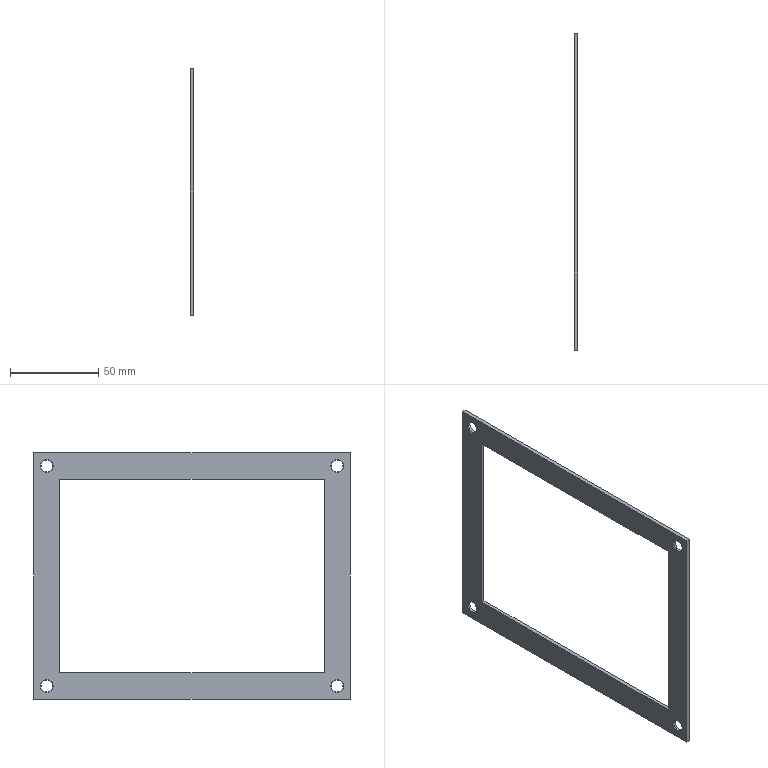Part | NX | 1 solid | 22 faces | box 2 x 180 x 140 mm | volume 17112 mm3 | plane 10 | cone 8 | cylinder 4 | commonest cylinder face diameters 6.6 x4
STEP:
#1=CARTESIAN_POINT('',(0.,-75.,-55.));
#2=VERTEX_POINT('',#1);
#3=CARTESIAN_POINT('',(0.,-75.,55.));
#4=VERTEX_POINT('',#3);
#5=CARTESIAN_POINT('',(0.,-75.,-55.));
#6=DIRECTION('',(0.,0.,1.));
#7=VECTOR('',#6,1.);
#8=LINE('',#5,#7);
#9=EDGE_CURVE('',#2,#4,#8,.T.);
#10=ORIENTED_EDGE('',*,*,#9,.T.);
#11=CARTESIAN_POINT('',(2.,-75.,55.));
#12=VERTEX_POINT('',#11);
#13=CARTESIAN_POINT('',(2.,-75.,55.));
#14=DIRECTION('',(-1.,0.,0.));
#15=VECTOR('',#14,1.);
#16=LINE('',#13,#15);
#17=EDGE_CURVE('',#12,#4,#16,.T.);
#18=ORIENTED_EDGE('',*,*,#17,.F.);
#19=CARTESIAN_POINT('',(2.,-75.,-55.));
#20=VERTEX_POINT('',#19);
#21=CARTESIAN_POINT('',(2.,-75.,-55.));
#22=DIRECTION('',(0.,0.,1.));
#23=VECTOR('',#22,1.);
#24=LINE('',#21,#23);
#25=EDGE_CURVE('',#20,#12,#24,.T.);
#26=ORIENTED_EDGE('',*,*,#25,.F.);
#27=CARTESIAN_POINT('',(2.,-75.,-55.));
#28=DIRECTION('',(-1.,0.,0.));
#29=VECTOR('',#28,1.);
#30=LINE('',#27,#29);
#31=EDGE_CURVE('',#20,#2,#30,.T.);
#32=ORIENTED_EDGE('',*,*,#31,.T.);
#33=EDGE_LOOP('',(#10,#18,#26,#32));
#34=FACE_OUTER_BOUND('',#33,.T.);
#35=CARTESIAN_POINT('',(2.,-75.,-55.));
#36=DIRECTION('',(0.,-1.,0.));
#37=DIRECTION('',(0.,0.,1.));
#38=AXIS2_PLACEMENT_3D('',#35,#36,#37);
#39=PLANE('',#38);
#40=ADVANCED_FACE('',(#34),#39,.F.);
#41=CARTESIAN_POINT('',(0.,75.,55.));
#42=VERTEX_POINT('',#41);
#43=CARTESIAN_POINT('',(0.,-75.,55.));
#44=DIRECTION('',(0.,1.,0.));
#45=VECTOR('',#44,1.);
#46=LINE('',#43,#45);
#47=EDGE_CURVE('',#4,#42,#46,.T.);
#48=ORIENTED_EDGE('',*,*,#47,.T.);
#49=CARTESIAN_POINT('',(2.,75.,55.));
#50=VERTEX_POINT('',#49);
#51=CARTESIAN_POINT('',(2.,75.,55.));
#52=DIRECTION('',(-1.,0.,0.));
#53=VECTOR('',#52,1.);
#54=LINE('',#51,#53);
#55=EDGE_CURVE('',#50,#42,#54,.T.);
#56=ORIENTED_EDGE('',*,*,#55,.F.);
#57=CARTESIAN_POINT('',(2.,-75.,55.));
#58=DIRECTION('',(0.,1.,0.));
#59=VECTOR('',#58,1.);
#60=LINE('',#57,#59);
#61=EDGE_CURVE('',#12,#50,#60,.T.);
#62=ORIENTED_EDGE('',*,*,#61,.F.);
#63=ORIENTED_EDGE('',*,*,#17,.T.);
#64=EDGE_LOOP('',(#48,#56,#62,#63));
#65=FACE_OUTER_BOUND('',#64,.T.);
#66=CARTESIAN_POINT('',(2.,-75.,55.));
#67=DIRECTION('',(0.,0.,1.));
#68=DIRECTION('',(0.,1.,0.));
#69=AXIS2_PLACEMENT_3D('',#66,#67,#68);
#70=PLANE('',#69);
#71=ADVANCED_FACE('',(#65),#70,.F.);
#72=CARTESIAN_POINT('',(0.,75.,-55.));
#73=VERTEX_POINT('',#72);
#74=CARTESIAN_POINT('',(0.,75.,55.));
#75=DIRECTION('',(0.,0.,-1.));
#76=VECTOR('',#75,1.);
#77=LINE('',#74,#76);
#78=EDGE_CURVE('',#42,#73,#77,.T.);
#79=ORIENTED_EDGE('',*,*,#78,.T.);
#80=CARTESIAN_POINT('',(2.,75.,-55.));
#81=VERTEX_POINT('',#80);
#82=CARTESIAN_POINT('',(2.,75.,-55.));
#83=DIRECTION('',(-1.,0.,0.));
#84=VECTOR('',#83,1.);
#85=LINE('',#82,#84);
#86=EDGE_CURVE('',#81,#73,#85,.T.);
#87=ORIENTED_EDGE('',*,*,#86,.F.);
#88=CARTESIAN_POINT('',(2.,75.,55.));
#89=DIRECTION('',(0.,0.,-1.));
#90=VECTOR('',#89,1.);
#91=LINE('',#88,#90);
#92=EDGE_CURVE('',#50,#81,#91,.T.);
#93=ORIENTED_EDGE('',*,*,#92,.F.);
#94=ORIENTED_EDGE('',*,*,#55,.T.);
#95=EDGE_LOOP('',(#79,#87,#93,#94));
#96=FACE_OUTER_BOUND('',#95,.T.);
#97=CARTESIAN_POINT('',(2.,75.,55.));
#98=DIRECTION('',(0.,1.,0.));
#99=DIRECTION('',(0.,0.,-1.));
#100=AXIS2_PLACEMENT_3D('',#97,#98,#99);
#101=PLANE('',#100);
#102=ADVANCED_FACE('',(#96),#101,.F.);
#103=CARTESIAN_POINT('',(0.,-90.,70.));
#104=VERTEX_POINT('',#103);
#105=CARTESIAN_POINT('',(0.,-90.,-70.));
#106=VERTEX_POINT('',#105);
#107=CARTESIAN_POINT('',(0.,-90.,70.));
#108=DIRECTION('',(0.,0.,-1.));
#109=VECTOR('',#108,1.);
#110=LINE('',#107,#109);
#111=EDGE_CURVE('',#104,#106,#110,.T.);
#112=ORIENTED_EDGE('',*,*,#111,.T.);
#113=CARTESIAN_POINT('',(2.,-90.,-70.));
#114=VERTEX_POINT('',#113);
#115=CARTESIAN_POINT('',(2.,-90.,-70.));
#116=DIRECTION('',(-1.,0.,0.));
#117=VECTOR('',#116,1.);
#118=LINE('',#115,#117);
#119=EDGE_CURVE('',#114,#106,#118,.T.);
#120=ORIENTED_EDGE('',*,*,#119,.F.);
#121=CARTESIAN_POINT('',(2.,-90.,70.));
#122=VERTEX_POINT('',#121);
#123=CARTESIAN_POINT('',(2.,-90.,70.));
#124=DIRECTION('',(0.,0.,-1.));
#125=VECTOR('',#124,1.);
#126=LINE('',#123,#125);
#127=EDGE_CURVE('',#122,#114,#126,.T.);
#128=ORIENTED_EDGE('',*,*,#127,.F.);
#129=CARTESIAN_POINT('',(2.,-90.,70.));
#130=DIRECTION('',(-1.,0.,0.));
#131=VECTOR('',#130,1.);
#132=LINE('',#129,#131);
#133=EDGE_CURVE('',#122,#104,#132,.T.);
#134=ORIENTED_EDGE('',*,*,#133,.T.);
#135=EDGE_LOOP('',(#112,#120,#128,#134));
#136=FACE_OUTER_BOUND('',#135,.T.);
#137=CARTESIAN_POINT('',(2.,-90.,70.));
#138=DIRECTION('',(0.,1.,0.));
#139=DIRECTION('',(0.,0.,-1.));
#140=AXIS2_PLACEMENT_3D('',#137,#138,#139);
#141=PLANE('',#140);
#142=ADVANCED_FACE('',(#136),#141,.F.);
#143=CARTESIAN_POINT('',(0.,90.,-70.));
#144=VERTEX_POINT('',#143);
#145=CARTESIAN_POINT('',(0.,-90.,-70.));
#146=DIRECTION('',(0.,1.,0.));
#147=VECTOR('',#146,1.);
#148=LINE('',#145,#147);
#149=EDGE_CURVE('',#106,#144,#148,.T.);
#150=ORIENTED_EDGE('',*,*,#149,.T.);
#151=CARTESIAN_POINT('',(2.,90.,-70.));
#152=VERTEX_POINT('',#151);
#153=CARTESIAN_POINT('',(2.,90.,-70.));
#154=DIRECTION('',(-1.,0.,0.));
#155=VECTOR('',#154,1.);
#156=LINE('',#153,#155);
#157=EDGE_CURVE('',#152,#144,#156,.T.);
#158=ORIENTED_EDGE('',*,*,#157,.F.);
#159=CARTESIAN_POINT('',(2.,-90.,-70.));
#160=DIRECTION('',(0.,1.,0.));
#161=VECTOR('',#160,1.);
#162=LINE('',#159,#161);
#163=EDGE_CURVE('',#114,#152,#162,.T.);
#164=ORIENTED_EDGE('',*,*,#163,.F.);
#165=ORIENTED_EDGE('',*,*,#119,.T.);
#166=EDGE_LOOP('',(#150,#158,#164,#165));
#167=FACE_OUTER_BOUND('',#166,.T.);
#168=CARTESIAN_POINT('',(2.,-90.,-70.));
#169=DIRECTION('',(0.,0.,1.));
#170=DIRECTION('',(0.,1.,0.));
#171=AXIS2_PLACEMENT_3D('',#168,#169,#170);
#172=PLANE('',#171);
#173=ADVANCED_FACE('',(#167),#172,.F.);
#174=CARTESIAN_POINT('',(0.,90.,70.));
#175=VERTEX_POINT('',#174);
#176=CARTESIAN_POINT('',(0.,90.,-70.));
#177=DIRECTION('',(0.,0.,1.));
#178=VECTOR('',#177,1.);
#179=LINE('',#176,#178);
#180=EDGE_CURVE('',#144,#175,#179,.T.);
#181=ORIENTED_EDGE('',*,*,#180,.T.);
#182=CARTESIAN_POINT('',(2.,90.,70.));
#183=VERTEX_POINT('',#182);
#184=CARTESIAN_POINT('',(2.,90.,70.));
#185=DIRECTION('',(-1.,0.,0.));
#186=VECTOR('',#185,1.);
#187=LINE('',#184,#186);
#188=EDGE_CURVE('',#183,#175,#187,.T.);
#189=ORIENTED_EDGE('',*,*,#188,.F.);
#190=CARTESIAN_POINT('',(2.,90.,-70.));
#191=DIRECTION('',(0.,0.,1.));
#192=VECTOR('',#191,1.);
#193=LINE('',#190,#192);
#194=EDGE_CURVE('',#152,#183,#193,.T.);
#195=ORIENTED_EDGE('',*,*,#194,.F.);
#196=ORIENTED_EDGE('',*,*,#157,.T.);
#197=EDGE_LOOP('',(#181,#189,#195,#196));
#198=FACE_OUTER_BOUND('',#197,.T.);
#199=CARTESIAN_POINT('',(2.,90.,-70.));
#200=DIRECTION('',(0.,-1.,0.));
#201=DIRECTION('',(0.,0.,1.));
#202=AXIS2_PLACEMENT_3D('',#199,#200,#201);
#203=PLANE('',#202);
#204=ADVANCED_FACE('',(#198),#203,.F.);
#205=CARTESIAN_POINT('',(0.,90.,70.));
#206=DIRECTION('',(0.,-1.,0.));
#207=VECTOR('',#206,1.);
#208=LINE('',#205,#207);
#209=EDGE_CURVE('',#175,#104,#208,.T.);
#210=ORIENTED_EDGE('',*,*,#209,.T.);
#211=ORIENTED_EDGE('',*,*,#133,.F.);
#212=CARTESIAN_POINT('',(2.,90.,70.));
#213=DIRECTION('',(0.,-1.,0.));
#214=VECTOR('',#213,1.);
#215=LINE('',#212,#214);
#216=EDGE_CURVE('',#183,#122,#215,.T.);
#217=ORIENTED_EDGE('',*,*,#216,.F.);
#218=ORIENTED_EDGE('',*,*,#188,.T.);
#219=EDGE_LOOP('',(#210,#211,#217,#218));
#220=FACE_OUTER_BOUND('',#219,.T.);
#221=CARTESIAN_POINT('',(2.,90.,70.));
#222=DIRECTION('',(0.,0.,-1.));
#223=DIRECTION('',(0.,-1.,0.));
#224=AXIS2_PLACEMENT_3D('',#221,#222,#223);
#225=PLANE('',#224);
#226=ADVANCED_FACE('',(#220),#225,.F.);
#227=CARTESIAN_POINT('',(0.,75.,-55.));
#228=DIRECTION('',(0.,-1.,0.));
#229=VECTOR('',#228,1.);
#230=LINE('',#227,#229);
#231=EDGE_CURVE('',#73,#2,#230,.T.);
#232=ORIENTED_EDGE('',*,*,#231,.T.);
#233=ORIENTED_EDGE('',*,*,#31,.F.);
#234=CARTESIAN_POINT('',(2.,75.,-55.));
#235=DIRECTION('',(0.,-1.,0.));
#236=VECTOR('',#235,1.);
#237=LINE('',#234,#236);
#238=EDGE_CURVE('',#81,#20,#237,.T.);
#239=ORIENTED_EDGE('',*,*,#238,.F.);
#240=ORIENTED_EDGE('',*,*,#86,.T.);
#241=EDGE_LOOP('',(#232,#233,#239,#240));
#242=FACE_OUTER_BOUND('',#241,.T.);
#243=CARTESIAN_POINT('',(2.,75.,-55.));
#244=DIRECTION('',(0.,0.,-1.));
#245=DIRECTION('',(0.,-1.,0.));
#246=AXIS2_PLACEMENT_3D('',#243,#244,#245);
#247=PLANE('',#246);
#248=ADVANCED_FACE('',(#242),#247,.F.);
#249=CARTESIAN_POINT('',(2.,82.5,58.8));
#250=VERTEX_POINT('',#249);
#251=CARTESIAN_POINT('',(2.,82.5,62.5));
#252=DIRECTION('',(-1.,0.,0.));
#253=DIRECTION('',(0.,0.,-1.));
#254=AXIS2_PLACEMENT_3D('',#251,#252,#253);
#255=CIRCLE('',#254,3.7);
#256=EDGE_CURVE('',#250,#250,#255,.T.);
#257=ORIENTED_EDGE('',*,*,#256,.T.);
#258=EDGE_LOOP('',(#257));
#259=FACE_BOUND('',#258,.T.);
#260=CARTESIAN_POINT('',(2.,82.5,-66.2));
#261=VERTEX_POINT('',#260);
#262=CARTESIAN_POINT('',(2.,82.5,-62.5));
#263=DIRECTION('',(-1.,0.,0.));
#264=DIRECTION('',(0.,0.,-1.));
#265=AXIS2_PLACEMENT_3D('',#262,#263,#264);
#266=CIRCLE('',#265,3.7);
#267=EDGE_CURVE('',#261,#261,#266,.T.);
#268=ORIENTED_EDGE('',*,*,#267,.T.);
#269=EDGE_LOOP('',(#268));
#270=FACE_BOUND('',#269,.T.);
#271=CARTESIAN_POINT('',(2.,-82.5,58.8));
#272=VERTEX_POINT('',#271);
#273=CARTESIAN_POINT('',(2.,-82.5,62.5));
#274=DIRECTION('',(-1.,0.,0.));
#275=DIRECTION('',(0.,0.,-1.));
#276=AXIS2_PLACEMENT_3D('',#273,#274,#275);
#277=CIRCLE('',#276,3.7);
#278=EDGE_CURVE('',#272,#272,#277,.T.);
#279=ORIENTED_EDGE('',*,*,#278,.T.);
#280=EDGE_LOOP('',(#279));
#281=FACE_BOUND('',#280,.T.);
#282=CARTESIAN_POINT('',(2.,-82.5,-66.2));
#283=VERTEX_POINT('',#282);
#284=CARTESIAN_POINT('',(2.,-82.5,-62.5));
#285=DIRECTION('',(-1.,0.,0.));
#286=DIRECTION('',(0.,0.,-1.));
#287=AXIS2_PLACEMENT_3D('',#284,#285,#286);
#288=CIRCLE('',#287,3.7);
#289=EDGE_CURVE('',#283,#283,#288,.T.);
#290=ORIENTED_EDGE('',*,*,#289,.T.);
#291=EDGE_LOOP('',(#290));
#292=FACE_BOUND('',#291,.T.);
#293=ORIENTED_EDGE('',*,*,#127,.T.);
#294=ORIENTED_EDGE('',*,*,#163,.T.);
#295=ORIENTED_EDGE('',*,*,#194,.T.);
#296=ORIENTED_EDGE('',*,*,#216,.T.);
#297=EDGE_LOOP('',(#293,#294,#295,#296));
#298=FACE_BOUND('',#297,.T.);
#299=ORIENTED_EDGE('',*,*,#25,.T.);
#300=ORIENTED_EDGE('',*,*,#61,.T.);
#301=ORIENTED_EDGE('',*,*,#92,.T.);
#302=ORIENTED_EDGE('',*,*,#238,.T.);
#303=EDGE_LOOP('',(#299,#300,#301,#302));
#304=FACE_BOUND('',#303,.T.);
#305=CARTESIAN_POINT('',(2.,0.,0.));
#306=DIRECTION('',(1.,0.,0.));
#307=DIRECTION('',(0.,0.,1.));
#308=AXIS2_PLACEMENT_3D('',#305,#306,#307);
#309=PLANE('',#308);
#310=ADVANCED_FACE('',(#259,#270,#281,#292,#298,#304),#309,.T.);
#311=CARTESIAN_POINT('',(0.,82.5,58.8));
#312=VERTEX_POINT('',#311);
#313=CARTESIAN_POINT('',(0.,82.5,62.5));
#314=DIRECTION('',(1.,0.,0.));
#315=DIRECTION('',(0.,0.,-1.));
#316=AXIS2_PLACEMENT_3D('',#313,#314,#315);
#317=CIRCLE('',#316,3.7);
#318=EDGE_CURVE('',#312,#312,#317,.T.);
#319=ORIENTED_EDGE('',*,*,#318,.T.);
#320=EDGE_LOOP('',(#319));
#321=FACE_BOUND('',#320,.T.);
#322=CARTESIAN_POINT('',(0.,82.5,-66.2));
#323=VERTEX_POINT('',#322);
#324=CARTESIAN_POINT('',(0.,82.5,-62.5));
#325=DIRECTION('',(1.,0.,0.));
#326=DIRECTION('',(0.,0.,-1.));
#327=AXIS2_PLACEMENT_3D('',#324,#325,#326);
#328=CIRCLE('',#327,3.7);
#329=EDGE_CURVE('',#323,#323,#328,.T.);
#330=ORIENTED_EDGE('',*,*,#329,.T.);
#331=EDGE_LOOP('',(#330));
#332=FACE_BOUND('',#331,.T.);
#333=CARTESIAN_POINT('',(0.,-82.5,58.8));
#334=VERTEX_POINT('',#333);
#335=CARTESIAN_POINT('',(0.,-82.5,62.5));
#336=DIRECTION('',(1.,0.,0.));
#337=DIRECTION('',(0.,0.,-1.));
#338=AXIS2_PLACEMENT_3D('',#335,#336,#337);
#339=CIRCLE('',#338,3.7);
#340=EDGE_CURVE('',#334,#334,#339,.T.);
#341=ORIENTED_EDGE('',*,*,#340,.T.);
#342=EDGE_LOOP('',(#341));
#343=FACE_BOUND('',#342,.T.);
#344=CARTESIAN_POINT('',(0.,-82.5,-66.2));
#345=VERTEX_POINT('',#344);
#346=CARTESIAN_POINT('',(0.,-82.5,-62.5));
#347=DIRECTION('',(1.,0.,0.));
#348=DIRECTION('',(0.,0.,-1.));
#349=AXIS2_PLACEMENT_3D('',#346,#347,#348);
#350=CIRCLE('',#349,3.7);
#351=EDGE_CURVE('',#345,#345,#350,.T.);
#352=ORIENTED_EDGE('',*,*,#351,.T.);
#353=EDGE_LOOP('',(#352));
#354=FACE_BOUND('',#353,.T.);
#355=ORIENTED_EDGE('',*,*,#111,.F.);
#356=ORIENTED_EDGE('',*,*,#209,.F.);
#357=ORIENTED_EDGE('',*,*,#180,.F.);
#358=ORIENTED_EDGE('',*,*,#149,.F.);
#359=EDGE_LOOP('',(#355,#356,#357,#358));
#360=FACE_BOUND('',#359,.T.);
#361=ORIENTED_EDGE('',*,*,#9,.F.);
#362=ORIENTED_EDGE('',*,*,#231,.F.);
#363=ORIENTED_EDGE('',*,*,#78,.F.);
#364=ORIENTED_EDGE('',*,*,#47,.F.);
#365=EDGE_LOOP('',(#361,#362,#363,#364));
#366=FACE_BOUND('',#365,.T.);
#367=CARTESIAN_POINT('',(0.,0.,0.));
#368=DIRECTION('',(1.,0.,0.));
#369=DIRECTION('',(0.,0.,1.));
#370=AXIS2_PLACEMENT_3D('',#367,#368,#369);
#371=PLANE('',#370);
#372=ADVANCED_FACE('',(#321,#332,#343,#354,#360,#366),#371,.F.);
#373=CARTESIAN_POINT('',(1.6,-82.5,-65.8));
#374=VERTEX_POINT('',#373);
#375=CARTESIAN_POINT('',(1.6,-82.5,-62.5));
#376=DIRECTION('',(1.,0.,0.));
#377=DIRECTION('',(0.,0.,-1.));
#378=AXIS2_PLACEMENT_3D('',#375,#376,#377);
#379=CIRCLE('',#378,3.3);
#380=EDGE_CURVE('',#374,#374,#379,.T.);
#381=ORIENTED_EDGE('',*,*,#380,.T.);
#382=EDGE_LOOP('',(#381));
#383=FACE_BOUND('',#382,.T.);
#384=CARTESIAN_POINT('',(0.4,-82.5,-65.8));
#385=VERTEX_POINT('',#384);
#386=CARTESIAN_POINT('',(0.4,-82.5,-62.5));
#387=DIRECTION('',(-1.,0.,0.));
#388=DIRECTION('',(0.,0.,-1.));
#389=AXIS2_PLACEMENT_3D('',#386,#387,#388);
#390=CIRCLE('',#389,3.3);
#391=EDGE_CURVE('',#385,#385,#390,.T.);
#392=ORIENTED_EDGE('',*,*,#391,.T.);
#393=EDGE_LOOP('',(#392));
#394=FACE_BOUND('',#393,.T.);
#395=CARTESIAN_POINT('',(0.,-82.5,-62.5));
#396=DIRECTION('',(1.,0.,0.));
#397=DIRECTION('',(0.,0.,1.));
#398=AXIS2_PLACEMENT_3D('',#395,#396,#397);
#399=CYLINDRICAL_SURFACE('',#398,3.3);
#400=ADVANCED_FACE('',(#383,#394),#399,.F.);
#401=ORIENTED_EDGE('',*,*,#391,.F.);
#402=EDGE_LOOP('',(#401));
#403=FACE_BOUND('',#402,.T.);
#404=ORIENTED_EDGE('',*,*,#351,.F.);
#405=EDGE_LOOP('',(#404));
#406=FACE_BOUND('',#405,.T.);
#407=CARTESIAN_POINT('',(0.,-82.5,-62.5));
#408=DIRECTION('',(-1.,0.,0.));
#409=DIRECTION('',(0.,0.,-1.));
#410=AXIS2_PLACEMENT_3D('',#407,#408,#409);
#411=CONICAL_SURFACE('',#410,3.7,45.);
#412=ADVANCED_FACE('',(#403,#406),#411,.F.);
#413=ORIENTED_EDGE('',*,*,#289,.F.);
#414=EDGE_LOOP('',(#413));
#415=FACE_BOUND('',#414,.T.);
#416=ORIENTED_EDGE('',*,*,#380,.F.);
#417=EDGE_LOOP('',(#416));
#418=FACE_BOUND('',#417,.T.);
#419=CARTESIAN_POINT('',(1.6,-82.5,-62.5));
#420=DIRECTION('',(1.,0.,0.));
#421=DIRECTION('',(0.,0.,1.));
#422=AXIS2_PLACEMENT_3D('',#419,#420,#421);
#423=CONICAL_SURFACE('',#422,3.3,45.);
#424=ADVANCED_FACE('',(#415,#418),#423,.F.);
#425=CARTESIAN_POINT('',(1.6,-82.5,59.2));
#426=VERTEX_POINT('',#425);
#427=CARTESIAN_POINT('',(1.6,-82.5,62.5));
#428=DIRECTION('',(1.,0.,0.));
#429=DIRECTION('',(0.,0.,-1.));
#430=AXIS2_PLACEMENT_3D('',#427,#428,#429);
#431=CIRCLE('',#430,3.3);
#432=EDGE_CURVE('',#426,#426,#431,.T.);
#433=ORIENTED_EDGE('',*,*,#432,.T.);
#434=EDGE_LOOP('',(#433));
#435=FACE_BOUND('',#434,.T.);
#436=CARTESIAN_POINT('',(0.4,-82.5,59.2));
#437=VERTEX_POINT('',#436);
#438=CARTESIAN_POINT('',(0.4,-82.5,62.5));
#439=DIRECTION('',(-1.,0.,0.));
#440=DIRECTION('',(0.,0.,-1.));
#441=AXIS2_PLACEMENT_3D('',#438,#439,#440);
#442=CIRCLE('',#441,3.3);
#443=EDGE_CURVE('',#437,#437,#442,.T.);
#444=ORIENTED_EDGE('',*,*,#443,.T.);
#445=EDGE_LOOP('',(#444));
#446=FACE_BOUND('',#445,.T.);
#447=CARTESIAN_POINT('',(0.,-82.5,62.5));
#448=DIRECTION('',(1.,0.,0.));
#449=DIRECTION('',(0.,0.,1.));
#450=AXIS2_PLACEMENT_3D('',#447,#448,#449);
#451=CYLINDRICAL_SURFACE('',#450,3.3);
#452=ADVANCED_FACE('',(#435,#446),#451,.F.);
#453=ORIENTED_EDGE('',*,*,#443,.F.);
#454=EDGE_LOOP('',(#453));
#455=FACE_BOUND('',#454,.T.);
#456=ORIENTED_EDGE('',*,*,#340,.F.);
#457=EDGE_LOOP('',(#456));
#458=FACE_BOUND('',#457,.T.);
#459=CARTESIAN_POINT('',(0.,-82.5,62.5));
#460=DIRECTION('',(-1.,0.,0.));
#461=DIRECTION('',(0.,0.,-1.));
#462=AXIS2_PLACEMENT_3D('',#459,#460,#461);
#463=CONICAL_SURFACE('',#462,3.7,45.);
#464=ADVANCED_FACE('',(#455,#458),#463,.F.);
#465=ORIENTED_EDGE('',*,*,#278,.F.);
#466=EDGE_LOOP('',(#465));
#467=FACE_BOUND('',#466,.T.);
#468=ORIENTED_EDGE('',*,*,#432,.F.);
#469=EDGE_LOOP('',(#468));
#470=FACE_BOUND('',#469,.T.);
#471=CARTESIAN_POINT('',(1.6,-82.5,62.5));
#472=DIRECTION('',(1.,0.,0.));
#473=DIRECTION('',(0.,0.,1.));
#474=AXIS2_PLACEMENT_3D('',#471,#472,#473);
#475=CONICAL_SURFACE('',#474,3.3,45.);
#476=ADVANCED_FACE('',(#467,#470),#475,.F.);
#477=CARTESIAN_POINT('',(1.6,82.5,-65.8));
#478=VERTEX_POINT('',#477);
#479=CARTESIAN_POINT('',(1.6,82.5,-62.5));
#480=DIRECTION('',(1.,0.,0.));
#481=DIRECTION('',(0.,0.,-1.));
#482=AXIS2_PLACEMENT_3D('',#479,#480,#481);
#483=CIRCLE('',#482,3.3);
#484=EDGE_CURVE('',#478,#478,#483,.T.);
#485=ORIENTED_EDGE('',*,*,#484,.T.);
#486=EDGE_LOOP('',(#485));
#487=FACE_BOUND('',#486,.T.);
#488=CARTESIAN_POINT('',(0.4,82.5,-65.8));
#489=VERTEX_POINT('',#488);
#490=CARTESIAN_POINT('',(0.4,82.5,-62.5));
#491=DIRECTION('',(-1.,0.,0.));
#492=DIRECTION('',(0.,0.,-1.));
#493=AXIS2_PLACEMENT_3D('',#490,#491,#492);
#494=CIRCLE('',#493,3.3);
#495=EDGE_CURVE('',#489,#489,#494,.T.);
#496=ORIENTED_EDGE('',*,*,#495,.T.);
#497=EDGE_LOOP('',(#496));
#498=FACE_BOUND('',#497,.T.);
#499=CARTESIAN_POINT('',(0.,82.5,-62.5));
#500=DIRECTION('',(1.,0.,0.));
#501=DIRECTION('',(0.,0.,1.));
#502=AXIS2_PLACEMENT_3D('',#499,#500,#501);
#503=CYLINDRICAL_SURFACE('',#502,3.3);
#504=ADVANCED_FACE('',(#487,#498),#503,.F.);
#505=ORIENTED_EDGE('',*,*,#495,.F.);
#506=EDGE_LOOP('',(#505));
#507=FACE_BOUND('',#506,.T.);
#508=ORIENTED_EDGE('',*,*,#329,.F.);
#509=EDGE_LOOP('',(#508));
#510=FACE_BOUND('',#509,.T.);
#511=CARTESIAN_POINT('',(0.,82.5,-62.5));
#512=DIRECTION('',(-1.,0.,0.));
#513=DIRECTION('',(0.,0.,-1.));
#514=AXIS2_PLACEMENT_3D('',#511,#512,#513);
#515=CONICAL_SURFACE('',#514,3.7,45.);
#516=ADVANCED_FACE('',(#507,#510),#515,.F.);
#517=ORIENTED_EDGE('',*,*,#267,.F.);
#518=EDGE_LOOP('',(#517));
#519=FACE_BOUND('',#518,.T.);
#520=ORIENTED_EDGE('',*,*,#484,.F.);
#521=EDGE_LOOP('',(#520));
#522=FACE_BOUND('',#521,.T.);
#523=CARTESIAN_POINT('',(1.6,82.5,-62.5));
#524=DIRECTION('',(1.,0.,0.));
#525=DIRECTION('',(0.,0.,1.));
#526=AXIS2_PLACEMENT_3D('',#523,#524,#525);
#527=CONICAL_SURFACE('',#526,3.3,45.);
#528=ADVANCED_FACE('',(#519,#522),#527,.F.);
#529=CARTESIAN_POINT('',(1.6,82.5,59.2));
#530=VERTEX_POINT('',#529);
#531=CARTESIAN_POINT('',(1.6,82.5,62.5));
#532=DIRECTION('',(1.,0.,0.));
#533=DIRECTION('',(0.,0.,-1.));
#534=AXIS2_PLACEMENT_3D('',#531,#532,#533);
#535=CIRCLE('',#534,3.3);
#536=EDGE_CURVE('',#530,#530,#535,.T.);
#537=ORIENTED_EDGE('',*,*,#536,.T.);
#538=EDGE_LOOP('',(#537));
#539=FACE_BOUND('',#538,.T.);
#540=CARTESIAN_POINT('',(0.4,82.5,59.2));
#541=VERTEX_POINT('',#540);
#542=CARTESIAN_POINT('',(0.4,82.5,62.5));
#543=DIRECTION('',(-1.,0.,0.));
#544=DIRECTION('',(0.,0.,-1.));
#545=AXIS2_PLACEMENT_3D('',#542,#543,#544);
#546=CIRCLE('',#545,3.3);
#547=EDGE_CURVE('',#541,#541,#546,.T.);
#548=ORIENTED_EDGE('',*,*,#547,.T.);
#549=EDGE_LOOP('',(#548));
#550=FACE_BOUND('',#549,.T.);
#551=CARTESIAN_POINT('',(0.,82.5,62.5));
#552=DIRECTION('',(1.,0.,0.));
#553=DIRECTION('',(0.,0.,1.));
#554=AXIS2_PLACEMENT_3D('',#551,#552,#553);
#555=CYLINDRICAL_SURFACE('',#554,3.3);
#556=ADVANCED_FACE('',(#539,#550),#555,.F.);
#557=ORIENTED_EDGE('',*,*,#547,.F.);
#558=EDGE_LOOP('',(#557));
#559=FACE_BOUND('',#558,.T.);
#560=ORIENTED_EDGE('',*,*,#318,.F.);
#561=EDGE_LOOP('',(#560));
#562=FACE_BOUND('',#561,.T.);
#563=CARTESIAN_POINT('',(0.,82.5,62.5));
#564=DIRECTION('',(-1.,0.,0.));
#565=DIRECTION('',(0.,0.,-1.));
#566=AXIS2_PLACEMENT_3D('',#563,#564,#565);
#567=CONICAL_SURFACE('',#566,3.7,45.);
#568=ADVANCED_FACE('',(#559,#562),#567,.F.);
#569=ORIENTED_EDGE('',*,*,#256,.F.);
#570=EDGE_LOOP('',(#569));
#571=FACE_BOUND('',#570,.T.);
#572=ORIENTED_EDGE('',*,*,#536,.F.);
#573=EDGE_LOOP('',(#572));
#574=FACE_BOUND('',#573,.T.);
#575=CARTESIAN_POINT('',(1.6,82.5,62.5));
#576=DIRECTION('',(1.,0.,0.));
#577=DIRECTION('',(0.,0.,1.));
#578=AXIS2_PLACEMENT_3D('',#575,#576,#577);
#579=CONICAL_SURFACE('',#578,3.3,45.);
#580=ADVANCED_FACE('',(#571,#574),#579,.F.);
#581=CLOSED_SHELL('',(#40,#71,#102,#142,#173,#204,#226,#248,#310,#372,#400,#412,#424,#452,#464,#476,#504,#516,#528,#556,#568,#580));
#582=MANIFOLD_SOLID_BREP('',#581);
#583=(LENGTH_UNIT()NAMED_UNIT(*)SI_UNIT(.MILLI.,.METRE.));
#584=UNCERTAINTY_MEASURE_WITH_UNIT(LENGTH_MEASURE(0.00002),#583,'','');
#585=(NAMED_UNIT(*)PLANE_ANGLE_UNIT()SI_UNIT($,.RADIAN.));
#586=PLANE_ANGLE_MEASURE_WITH_UNIT(PLANE_ANGLE_MEASURE(0.01745),#585);
#587=DIMENSIONAL_EXPONENTS(0.,0.,0.,0.,0.,0.,0.);
#588=(CONVERSION_BASED_UNIT('DEGREE',#586)NAMED_UNIT(#587)PLANE_ANGLE_UNIT());
#589=(NAMED_UNIT(*)SI_UNIT($,.STERADIAN.)SOLID_ANGLE_UNIT());
#590=(GEOMETRIC_REPRESENTATION_CONTEXT(3)GLOBAL_UNCERTAINTY_ASSIGNED_CONTEXT((#584))GLOBAL_UNIT_ASSIGNED_CONTEXT((#583,#588,#589))REPRESENTATION_CONTEXT('',''));
#591=ADVANCED_BREP_SHAPE_REPRESENTATION('',(#582),#590);